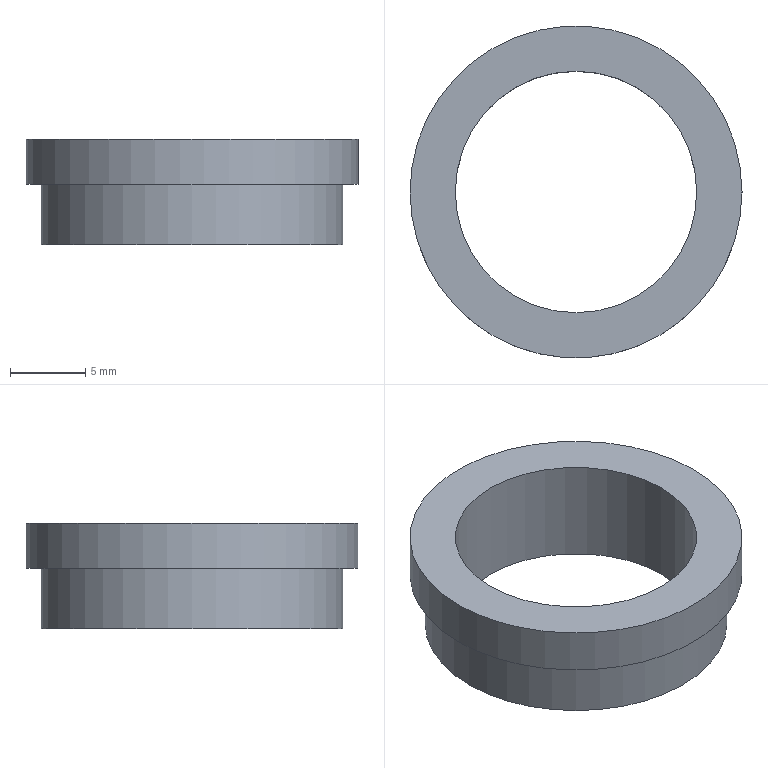Part | STEP file | 1-56.5 | 1 solid | 6 faces | box 22 x 22 x 7 mm | volume 989.602 mm3 | plane 3 | cylinder 3 | commonest cylinder face diameters 16 x1 20 x1 22 x1
STEP:
#1=CARTESIAN_POINT('',(0.,0.,0.));
#2=DIRECTION('',(0.,0.,1.));
#3=DIRECTION('',(1.,0.,0.));
#4=AXIS2_PLACEMENT_3D('',#1,#2,#3);
#5=CARTESIAN_POINT('',(10.,0.,-4.));
#6=VERTEX_POINT('',#5);
#7=CARTESIAN_POINT('',(0.,0.,-4.));
#8=DIRECTION('',(0.,0.,1.));
#9=DIRECTION('',(1.,0.,0.));
#10=AXIS2_PLACEMENT_3D('',#7,#8,#9);
#11=CIRCLE('',#10,10.);
#12=CARTESIAN_POINT('',(-2.679,0.,-4.));
#13=DIRECTION('',(0.,0.,1.));
#14=DIRECTION('',(1.,0.,0.));
#15=AXIS2_PLACEMENT_3D('',#12,#13,#14);
#16=PLANE('',#15);
#17=CARTESIAN_POINT('',(2.679,0.));
#18=DIRECTION('',(1.,0.));
#19=AXIS2_PLACEMENT_2D('',#17,#18);
#20=CIRCLE('',#19,10.);
#21=(GEOMETRIC_REPRESENTATION_CONTEXT(2)PARAMETRIC_REPRESENTATION_CONTEXT()REPRESENTATION_CONTEXT('',''));
#22=DEFINITIONAL_REPRESENTATION('',(#20),#21);
#23=PCURVE('',#16,#22);
#24=CARTESIAN_POINT('',(0.,0.,0.));
#25=DIRECTION('',(0.,0.,-1.));
#26=DIRECTION('',(1.,0.,0.));
#27=AXIS2_PLACEMENT_3D('',#24,#25,#26);
#28=CYLINDRICAL_SURFACE('',#27,10.);
#29=CARTESIAN_POINT('',(6.283,4.));
#30=DIRECTION('',(-1.,0.));
#31=VECTOR('',#30,1.);
#32=LINE('',#29,#31);
#33=(GEOMETRIC_REPRESENTATION_CONTEXT(2)PARAMETRIC_REPRESENTATION_CONTEXT()REPRESENTATION_CONTEXT('',''));
#34=DEFINITIONAL_REPRESENTATION('',(#32),#33);
#35=PCURVE('',#28,#34);
#36=SURFACE_CURVE('',#11,(#23,#35),.PCURVE_S1.);
#37=EDGE_CURVE('',#6,#6,#36,.T.);
#38=ORIENTED_EDGE('',*,*,#37,.T.);
#39=EDGE_LOOP('',(#38));
#40=FACE_BOUND('',#39,.F.);
#41=CARTESIAN_POINT('',(8.,0.,-4.));
#42=VERTEX_POINT('',#41);
#43=CARTESIAN_POINT('',(0.,0.,-4.));
#44=DIRECTION('',(0.,0.,-1.));
#45=DIRECTION('',(1.,0.,0.));
#46=AXIS2_PLACEMENT_3D('',#43,#44,#45);
#47=CIRCLE('',#46,8.);
#48=CARTESIAN_POINT('',(10.679,0.));
#49=CARTESIAN_POINT('',(10.679,-13.856));
#50=CARTESIAN_POINT('',(-1.321,-6.928));
#51=CARTESIAN_POINT('',(-13.321,0.));
#52=CARTESIAN_POINT('',(-1.321,6.928));
#53=CARTESIAN_POINT('',(10.679,13.856));
#54=CARTESIAN_POINT('',(10.679,0.));
#55=(BOUNDED_CURVE()B_SPLINE_CURVE(2,(#48,#49,#50,#51,#52,#53,#54),.UNSPECIFIED.,.T.,.F.)B_SPLINE_CURVE_WITH_KNOTS((1,2,2,2,2,1),(-2.094,0.,2.094,4.189,6.283,8.378),.UNSPECIFIED.)CURVE()GEOMETRIC_REPRESENTATION_ITEM()RATIONAL_B_SPLINE_CURVE((1.,0.5,1.,0.5,1.,0.5,1.))REPRESENTATION_ITEM(''));
#56=(GEOMETRIC_REPRESENTATION_CONTEXT(2)PARAMETRIC_REPRESENTATION_CONTEXT()REPRESENTATION_CONTEXT('',''));
#57=DEFINITIONAL_REPRESENTATION('',(#55),#56);
#58=PCURVE('',#16,#57);
#59=CARTESIAN_POINT('',(0.,0.,3.));
#60=DIRECTION('',(0.,0.,-1.));
#61=DIRECTION('',(1.,0.,0.));
#62=AXIS2_PLACEMENT_3D('',#59,#60,#61);
#63=CYLINDRICAL_SURFACE('',#62,8.);
#64=CARTESIAN_POINT('',(0.,7.));
#65=DIRECTION('',(1.,0.));
#66=VECTOR('',#65,1.);
#67=LINE('',#64,#66);
#68=(GEOMETRIC_REPRESENTATION_CONTEXT(2)PARAMETRIC_REPRESENTATION_CONTEXT()REPRESENTATION_CONTEXT('',''));
#69=DEFINITIONAL_REPRESENTATION('',(#67),#68);
#70=PCURVE('',#63,#69);
#71=SURFACE_CURVE('',#47,(#58,#70),.PCURVE_S1.);
#72=EDGE_CURVE('',#42,#42,#71,.T.);
#73=ORIENTED_EDGE('',*,*,#72,.T.);
#74=EDGE_LOOP('',(#73));
#75=FACE_BOUND('',#74,.F.);
#76=ADVANCED_FACE('',(#40,#75),#16,.F.);
#77=CARTESIAN_POINT('',(10.,0.,0.));
#78=VERTEX_POINT('',#77);
#79=CARTESIAN_POINT('',(10.,0.,0.));
#80=DIRECTION('',(0.,0.,-1.));
#81=VECTOR('',#80,1.);
#82=LINE('',#79,#81);
#83=CARTESIAN_POINT('',(6.283,0.));
#84=DIRECTION('',(0.,1.));
#85=VECTOR('',#84,1.);
#86=LINE('',#83,#85);
#87=(GEOMETRIC_REPRESENTATION_CONTEXT(2)PARAMETRIC_REPRESENTATION_CONTEXT()REPRESENTATION_CONTEXT('',''));
#88=DEFINITIONAL_REPRESENTATION('',(#86),#87);
#89=PCURVE('',#28,#88);
#90=CARTESIAN_POINT('',(0.,0.));
#91=DIRECTION('',(0.,1.));
#92=VECTOR('',#91,1.);
#93=LINE('',#90,#92);
#94=(GEOMETRIC_REPRESENTATION_CONTEXT(2)PARAMETRIC_REPRESENTATION_CONTEXT()REPRESENTATION_CONTEXT('',''));
#95=DEFINITIONAL_REPRESENTATION('',(#93),#94);
#96=PCURVE('',#28,#95);
#97=SEAM_CURVE('',#82,(#89,#96),.PCURVE_S1.);
#98=EDGE_CURVE('',#78,#6,#97,.T.);
#99=ORIENTED_EDGE('',*,*,#98,.T.);
#100=ORIENTED_EDGE('',*,*,#37,.T.);
#101=ORIENTED_EDGE('',*,*,#98,.F.);
#102=CARTESIAN_POINT('',(0.,0.,0.));
#103=DIRECTION('',(0.,0.,1.));
#104=DIRECTION('',(1.,0.,0.));
#105=AXIS2_PLACEMENT_3D('',#102,#103,#104);
#106=CIRCLE('',#105,10.);
#107=CARTESIAN_POINT('',(6.283,0.));
#108=DIRECTION('',(-1.,0.));
#109=VECTOR('',#108,1.);
#110=LINE('',#107,#109);
#111=(GEOMETRIC_REPRESENTATION_CONTEXT(2)PARAMETRIC_REPRESENTATION_CONTEXT()REPRESENTATION_CONTEXT('',''));
#112=DEFINITIONAL_REPRESENTATION('',(#110),#111);
#113=PCURVE('',#28,#112);
#114=CARTESIAN_POINT('',(-2.947,0.,0.));
#115=DIRECTION('',(0.,0.,1.));
#116=DIRECTION('',(1.,0.,0.));
#117=AXIS2_PLACEMENT_3D('',#114,#115,#116);
#118=PLANE('',#117);
#119=CARTESIAN_POINT('',(2.947,0.));
#120=DIRECTION('',(1.,0.));
#121=AXIS2_PLACEMENT_2D('',#119,#120);
#122=CIRCLE('',#121,10.);
#123=(GEOMETRIC_REPRESENTATION_CONTEXT(2)PARAMETRIC_REPRESENTATION_CONTEXT()REPRESENTATION_CONTEXT('',''));
#124=DEFINITIONAL_REPRESENTATION('',(#122),#123);
#125=PCURVE('',#118,#124);
#126=SURFACE_CURVE('',#106,(#113,#125),.PCURVE_S1.);
#127=EDGE_CURVE('',#78,#78,#126,.T.);
#128=ORIENTED_EDGE('',*,*,#127,.F.);
#129=EDGE_LOOP('',(#99,#100,#101,#128));
#130=FACE_BOUND('',#129,.T.);
#131=ADVANCED_FACE('',(#130),#28,.T.);
#132=ORIENTED_EDGE('',*,*,#72,.F.);
#133=CARTESIAN_POINT('',(8.,0.,3.));
#134=VERTEX_POINT('',#133);
#135=CARTESIAN_POINT('',(8.,0.,-4.));
#136=DIRECTION('',(0.,0.,1.));
#137=VECTOR('',#136,1.);
#138=LINE('',#135,#137);
#139=CARTESIAN_POINT('',(0.,7.));
#140=DIRECTION('',(0.,-1.));
#141=VECTOR('',#140,1.);
#142=LINE('',#139,#141);
#143=(GEOMETRIC_REPRESENTATION_CONTEXT(2)PARAMETRIC_REPRESENTATION_CONTEXT()REPRESENTATION_CONTEXT('',''));
#144=DEFINITIONAL_REPRESENTATION('',(#142),#143);
#145=PCURVE('',#63,#144);
#146=CARTESIAN_POINT('',(6.283,7.));
#147=DIRECTION('',(0.,-1.));
#148=VECTOR('',#147,1.);
#149=LINE('',#146,#148);
#150=(GEOMETRIC_REPRESENTATION_CONTEXT(2)PARAMETRIC_REPRESENTATION_CONTEXT()REPRESENTATION_CONTEXT('',''));
#151=DEFINITIONAL_REPRESENTATION('',(#149),#150);
#152=PCURVE('',#63,#151);
#153=SEAM_CURVE('',#138,(#145,#152),.PCURVE_S1.);
#154=EDGE_CURVE('',#42,#134,#153,.T.);
#155=ORIENTED_EDGE('',*,*,#154,.T.);
#156=CARTESIAN_POINT('',(0.,0.,3.));
#157=DIRECTION('',(0.,0.,-1.));
#158=DIRECTION('',(1.,0.,0.));
#159=AXIS2_PLACEMENT_3D('',#156,#157,#158);
#160=CIRCLE('',#159,8.);
#161=CARTESIAN_POINT('',(0.,0.));
#162=DIRECTION('',(1.,0.));
#163=VECTOR('',#162,1.);
#164=LINE('',#161,#163);
#165=(GEOMETRIC_REPRESENTATION_CONTEXT(2)PARAMETRIC_REPRESENTATION_CONTEXT()REPRESENTATION_CONTEXT('',''));
#166=DEFINITIONAL_REPRESENTATION('',(#164),#165);
#167=PCURVE('',#63,#166);
#168=CARTESIAN_POINT('',(-2.947,0.,3.));
#169=DIRECTION('',(0.,0.,1.));
#170=DIRECTION('',(1.,0.,0.));
#171=AXIS2_PLACEMENT_3D('',#168,#169,#170);
#172=PLANE('',#171);
#173=CARTESIAN_POINT('',(10.947,0.));
#174=CARTESIAN_POINT('',(10.947,-13.856));
#175=CARTESIAN_POINT('',(-1.053,-6.928));
#176=CARTESIAN_POINT('',(-13.053,0.));
#177=CARTESIAN_POINT('',(-1.053,6.928));
#178=CARTESIAN_POINT('',(10.947,13.856));
#179=CARTESIAN_POINT('',(10.947,0.));
#180=(BOUNDED_CURVE()B_SPLINE_CURVE(2,(#173,#174,#175,#176,#177,#178,#179),.UNSPECIFIED.,.T.,.F.)B_SPLINE_CURVE_WITH_KNOTS((1,2,2,2,2,1),(-2.094,0.,2.094,4.189,6.283,8.378),.UNSPECIFIED.)CURVE()GEOMETRIC_REPRESENTATION_ITEM()RATIONAL_B_SPLINE_CURVE((1.,0.5,1.,0.5,1.,0.5,1.))REPRESENTATION_ITEM(''));
#181=(GEOMETRIC_REPRESENTATION_CONTEXT(2)PARAMETRIC_REPRESENTATION_CONTEXT()REPRESENTATION_CONTEXT('',''));
#182=DEFINITIONAL_REPRESENTATION('',(#180),#181);
#183=PCURVE('',#172,#182);
#184=SURFACE_CURVE('',#160,(#167,#183),.PCURVE_S1.);
#185=EDGE_CURVE('',#134,#134,#184,.T.);
#186=ORIENTED_EDGE('',*,*,#185,.T.);
#187=ORIENTED_EDGE('',*,*,#154,.F.);
#188=EDGE_LOOP('',(#132,#155,#186,#187));
#189=FACE_BOUND('',#188,.F.);
#190=ADVANCED_FACE('',(#189),#63,.F.);
#191=CARTESIAN_POINT('',(11.,0.,0.));
#192=VERTEX_POINT('',#191);
#193=CARTESIAN_POINT('',(0.,0.,0.));
#194=DIRECTION('',(0.,0.,1.));
#195=DIRECTION('',(1.,0.,0.));
#196=AXIS2_PLACEMENT_3D('',#193,#194,#195);
#197=CIRCLE('',#196,11.);
#198=CARTESIAN_POINT('',(2.947,0.));
#199=DIRECTION('',(1.,0.));
#200=AXIS2_PLACEMENT_2D('',#198,#199);
#201=CIRCLE('',#200,11.);
#202=(GEOMETRIC_REPRESENTATION_CONTEXT(2)PARAMETRIC_REPRESENTATION_CONTEXT()REPRESENTATION_CONTEXT('',''));
#203=DEFINITIONAL_REPRESENTATION('',(#201),#202);
#204=PCURVE('',#118,#203);
#205=CARTESIAN_POINT('',(0.,0.,0.));
#206=DIRECTION('',(0.,0.,1.));
#207=DIRECTION('',(1.,0.,0.));
#208=AXIS2_PLACEMENT_3D('',#205,#206,#207);
#209=CYLINDRICAL_SURFACE('',#208,11.);
#210=CARTESIAN_POINT('',(0.,0.));
#211=DIRECTION('',(1.,0.));
#212=VECTOR('',#211,1.);
#213=LINE('',#210,#212);
#214=(GEOMETRIC_REPRESENTATION_CONTEXT(2)PARAMETRIC_REPRESENTATION_CONTEXT()REPRESENTATION_CONTEXT('',''));
#215=DEFINITIONAL_REPRESENTATION('',(#213),#214);
#216=PCURVE('',#209,#215);
#217=SURFACE_CURVE('',#197,(#204,#216),.PCURVE_S1.);
#218=EDGE_CURVE('',#192,#192,#217,.T.);
#219=ORIENTED_EDGE('',*,*,#218,.T.);
#220=EDGE_LOOP('',(#219));
#221=FACE_BOUND('',#220,.F.);
#222=ORIENTED_EDGE('',*,*,#127,.F.);
#223=EDGE_LOOP('',(#222));
#224=FACE_BOUND('',#223,.F.);
#225=ADVANCED_FACE('',(#221,#224),#118,.F.);
#226=ORIENTED_EDGE('',*,*,#218,.T.);
#227=CARTESIAN_POINT('',(11.,0.,3.));
#228=VERTEX_POINT('',#227);
#229=CARTESIAN_POINT('',(11.,0.,0.));
#230=DIRECTION('',(0.,0.,1.));
#231=VECTOR('',#230,1.);
#232=LINE('',#229,#231);
#233=CARTESIAN_POINT('',(6.283,0.));
#234=DIRECTION('',(0.,1.));
#235=VECTOR('',#234,1.);
#236=LINE('',#233,#235);
#237=(GEOMETRIC_REPRESENTATION_CONTEXT(2)PARAMETRIC_REPRESENTATION_CONTEXT()REPRESENTATION_CONTEXT('',''));
#238=DEFINITIONAL_REPRESENTATION('',(#236),#237);
#239=PCURVE('',#209,#238);
#240=CARTESIAN_POINT('',(0.,0.));
#241=DIRECTION('',(0.,1.));
#242=VECTOR('',#241,1.);
#243=LINE('',#240,#242);
#244=(GEOMETRIC_REPRESENTATION_CONTEXT(2)PARAMETRIC_REPRESENTATION_CONTEXT()REPRESENTATION_CONTEXT('',''));
#245=DEFINITIONAL_REPRESENTATION('',(#243),#244);
#246=PCURVE('',#209,#245);
#247=SEAM_CURVE('',#232,(#239,#246),.PCURVE_S1.);
#248=EDGE_CURVE('',#192,#228,#247,.T.);
#249=ORIENTED_EDGE('',*,*,#248,.T.);
#250=CARTESIAN_POINT('',(0.,0.,3.));
#251=DIRECTION('',(0.,0.,1.));
#252=DIRECTION('',(1.,0.,0.));
#253=AXIS2_PLACEMENT_3D('',#250,#251,#252);
#254=CIRCLE('',#253,11.);
#255=CARTESIAN_POINT('',(0.,3.));
#256=DIRECTION('',(1.,0.));
#257=VECTOR('',#256,1.);
#258=LINE('',#255,#257);
#259=(GEOMETRIC_REPRESENTATION_CONTEXT(2)PARAMETRIC_REPRESENTATION_CONTEXT()REPRESENTATION_CONTEXT('',''));
#260=DEFINITIONAL_REPRESENTATION('',(#258),#259);
#261=PCURVE('',#209,#260);
#262=CARTESIAN_POINT('',(2.947,0.));
#263=DIRECTION('',(1.,0.));
#264=AXIS2_PLACEMENT_2D('',#262,#263);
#265=CIRCLE('',#264,11.);
#266=(GEOMETRIC_REPRESENTATION_CONTEXT(2)PARAMETRIC_REPRESENTATION_CONTEXT()REPRESENTATION_CONTEXT('',''));
#267=DEFINITIONAL_REPRESENTATION('',(#265),#266);
#268=PCURVE('',#172,#267);
#269=SURFACE_CURVE('',#254,(#261,#268),.PCURVE_S1.);
#270=EDGE_CURVE('',#228,#228,#269,.T.);
#271=ORIENTED_EDGE('',*,*,#270,.F.);
#272=ORIENTED_EDGE('',*,*,#248,.F.);
#273=EDGE_LOOP('',(#226,#249,#271,#272));
#274=FACE_BOUND('',#273,.T.);
#275=ADVANCED_FACE('',(#274),#209,.T.);
#276=ORIENTED_EDGE('',*,*,#270,.T.);
#277=EDGE_LOOP('',(#276));
#278=FACE_BOUND('',#277,.T.);
#279=ORIENTED_EDGE('',*,*,#185,.T.);
#280=EDGE_LOOP('',(#279));
#281=FACE_BOUND('',#280,.T.);
#282=ADVANCED_FACE('',(#278,#281),#172,.T.);
#283=CLOSED_SHELL('',(#76,#131,#190,#225,#275,#282));
#284=MANIFOLD_SOLID_BREP('',#283);
#285=(LENGTH_UNIT()NAMED_UNIT(*)SI_UNIT(.MILLI.,.METRE.));
#286=UNCERTAINTY_MEASURE_WITH_UNIT(LENGTH_MEASURE(0.0000001),#285,'','');
#287=(NAMED_UNIT(*)PLANE_ANGLE_UNIT()SI_UNIT($,.RADIAN.));
#288=(NAMED_UNIT(*)SI_UNIT($,.STERADIAN.)SOLID_ANGLE_UNIT());
#289=(GEOMETRIC_REPRESENTATION_CONTEXT(3)GLOBAL_UNCERTAINTY_ASSIGNED_CONTEXT((#286))GLOBAL_UNIT_ASSIGNED_CONTEXT((#285,#287,#288))REPRESENTATION_CONTEXT('',''));
#290=ADVANCED_BREP_SHAPE_REPRESENTATION('',(#4,#284),#289);